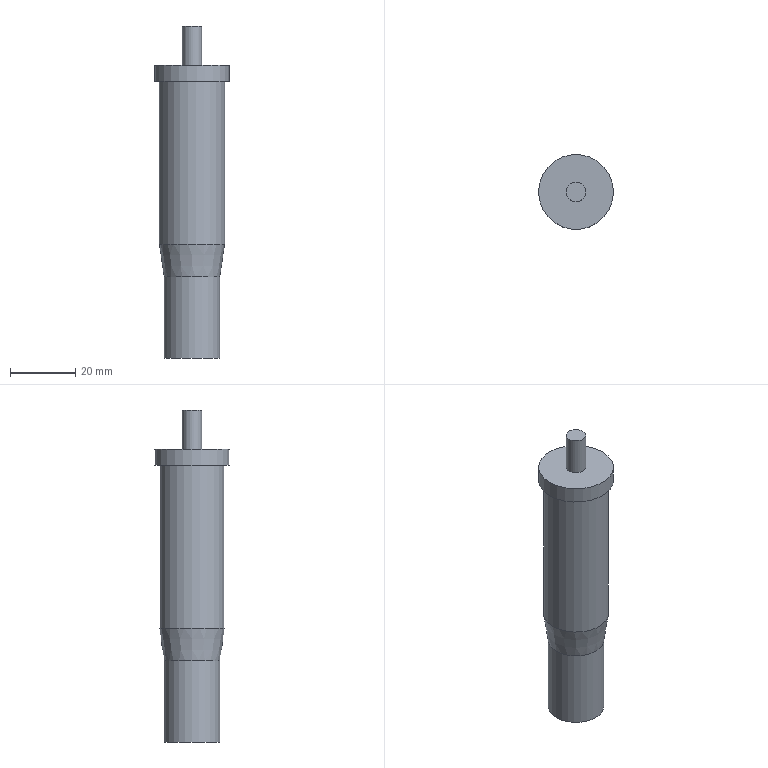Part | NX | features solid 2 | 1 solid | 9 faces | box 23 x 23 x 102 mm | volume 26574 mm3 | plane 4 | cylinder 4 | cone 1 | commonest cylinder face diameters 6 x1 17.1 x1 20 x1 23 x1
STEP:
#1=CARTESIAN_POINT('',(512.992,-137.822,-16.));
#2=VERTEX_POINT('',#1);
#3=CARTESIAN_POINT('',(521.542,-137.822,-16.));
#4=DIRECTION('',(0.,0.,-1.));
#5=DIRECTION('',(-1.,0.,0.));
#6=AXIS2_PLACEMENT_3D('',#3,#4,#5);
#7=CIRCLE('',#6,8.55);
#8=EDGE_CURVE('',#2,#2,#7,.T.);
#9=ORIENTED_EDGE('',*,*,#8,.T.);
#10=EDGE_LOOP('',(#9));
#11=FACE_BOUND('',#10,.T.);
#12=CARTESIAN_POINT('',(521.542,-137.822,-16.));
#13=DIRECTION('',(0.,0.,-1.));
#14=DIRECTION('',(1.,0.,0.));
#15=AXIS2_PLACEMENT_3D('',#12,#13,#14);
#16=PLANE('',#15);
#17=ADVANCED_FACE('',(#11),#16,.T.);
#18=CARTESIAN_POINT('',(512.992,-137.822,9.));
#19=VERTEX_POINT('',#18);
#20=CARTESIAN_POINT('',(521.542,-137.822,9.));
#21=DIRECTION('',(0.,0.,-1.));
#22=DIRECTION('',(-1.,0.,0.));
#23=AXIS2_PLACEMENT_3D('',#20,#21,#22);
#24=CIRCLE('',#23,8.55);
#25=EDGE_CURVE('',#19,#19,#24,.T.);
#26=ORIENTED_EDGE('',*,*,#25,.T.);
#27=EDGE_LOOP('',(#26));
#28=FACE_BOUND('',#27,.T.);
#29=ORIENTED_EDGE('',*,*,#8,.F.);
#30=EDGE_LOOP('',(#29));
#31=FACE_BOUND('',#30,.T.);
#32=CARTESIAN_POINT('',(521.542,-137.822,-16.));
#33=DIRECTION('',(0.,0.,1.));
#34=DIRECTION('',(-1.,0.,0.));
#35=AXIS2_PLACEMENT_3D('',#32,#33,#34);
#36=CYLINDRICAL_SURFACE('',#35,8.55);
#37=ADVANCED_FACE('',(#28,#31),#36,.T.);
#38=ORIENTED_EDGE('',*,*,#25,.F.);
#39=EDGE_LOOP('',(#38));
#40=FACE_BOUND('',#39,.T.);
#41=CARTESIAN_POINT('',(511.542,-137.822,19.));
#42=VERTEX_POINT('',#41);
#43=CARTESIAN_POINT('',(521.542,-137.822,19.));
#44=DIRECTION('',(0.,0.,-1.));
#45=DIRECTION('',(-1.,0.,0.));
#46=AXIS2_PLACEMENT_3D('',#43,#44,#45);
#47=CIRCLE('',#46,10.);
#48=EDGE_CURVE('',#42,#42,#47,.T.);
#49=ORIENTED_EDGE('',*,*,#48,.T.);
#50=EDGE_LOOP('',(#49));
#51=FACE_BOUND('',#50,.T.);
#52=CARTESIAN_POINT('',(521.542,-137.822,9.));
#53=DIRECTION('',(0.,0.,1.));
#54=DIRECTION('',(-1.,0.,0.));
#55=AXIS2_PLACEMENT_3D('',#52,#53,#54);
#56=CONICAL_SURFACE('',#55,8.55,0.144);
#57=ADVANCED_FACE('',(#40,#51),#56,.T.);
#58=CARTESIAN_POINT('',(531.542,-137.822,69.));
#59=VERTEX_POINT('',#58);
#60=CARTESIAN_POINT('',(521.542,-137.822,69.));
#61=DIRECTION('',(0.,0.,1.));
#62=DIRECTION('',(1.,0.,0.));
#63=AXIS2_PLACEMENT_3D('',#60,#61,#62);
#64=CIRCLE('',#63,10.);
#65=EDGE_CURVE('',#59,#59,#64,.F.);
#66=ORIENTED_EDGE('',*,*,#65,.T.);
#67=EDGE_LOOP('',(#66));
#68=FACE_BOUND('',#67,.T.);
#69=ORIENTED_EDGE('',*,*,#48,.F.);
#70=EDGE_LOOP('',(#69));
#71=FACE_BOUND('',#70,.T.);
#72=CARTESIAN_POINT('',(521.542,-137.822,19.));
#73=DIRECTION('',(0.,0.,1.));
#74=DIRECTION('',(-1.,0.,0.));
#75=AXIS2_PLACEMENT_3D('',#72,#73,#74);
#76=CYLINDRICAL_SURFACE('',#75,10.);
#77=ADVANCED_FACE('',(#68,#71),#76,.T.);
#78=CARTESIAN_POINT('',(518.542,-137.822,74.));
#79=VERTEX_POINT('',#78);
#80=CARTESIAN_POINT('',(521.542,-137.822,74.));
#81=DIRECTION('',(0.,0.,-1.));
#82=DIRECTION('',(-1.,0.,0.));
#83=AXIS2_PLACEMENT_3D('',#80,#81,#82);
#84=CIRCLE('',#83,3.);
#85=EDGE_CURVE('',#79,#79,#84,.T.);
#86=ORIENTED_EDGE('',*,*,#85,.T.);
#87=EDGE_LOOP('',(#86));
#88=FACE_BOUND('',#87,.T.);
#89=CARTESIAN_POINT('',(533.042,-137.822,74.));
#90=VERTEX_POINT('',#89);
#91=CARTESIAN_POINT('',(521.542,-137.822,74.));
#92=DIRECTION('',(0.,0.,1.));
#93=DIRECTION('',(1.,0.,0.));
#94=AXIS2_PLACEMENT_3D('',#91,#92,#93);
#95=CIRCLE('',#94,11.5);
#96=EDGE_CURVE('',#90,#90,#95,.T.);
#97=ORIENTED_EDGE('',*,*,#96,.T.);
#98=EDGE_LOOP('',(#97));
#99=FACE_BOUND('',#98,.T.);
#100=CARTESIAN_POINT('',(521.542,-137.822,74.));
#101=DIRECTION('',(0.,0.,1.));
#102=DIRECTION('',(-1.,0.,0.));
#103=AXIS2_PLACEMENT_3D('',#100,#101,#102);
#104=PLANE('',#103);
#105=ADVANCED_FACE('',(#88,#99),#104,.T.);
#106=ORIENTED_EDGE('',*,*,#65,.F.);
#107=EDGE_LOOP('',(#106));
#108=FACE_BOUND('',#107,.T.);
#109=CARTESIAN_POINT('',(510.042,-137.822,69.));
#110=VERTEX_POINT('',#109);
#111=CARTESIAN_POINT('',(521.542,-137.822,69.));
#112=DIRECTION('',(0.,0.,-1.));
#113=DIRECTION('',(-1.,0.,0.));
#114=AXIS2_PLACEMENT_3D('',#111,#112,#113);
#115=CIRCLE('',#114,11.5);
#116=EDGE_CURVE('',#110,#110,#115,.T.);
#117=ORIENTED_EDGE('',*,*,#116,.T.);
#118=EDGE_LOOP('',(#117));
#119=FACE_BOUND('',#118,.T.);
#120=CARTESIAN_POINT('',(521.542,-137.822,69.));
#121=DIRECTION('',(0.,0.,-1.));
#122=DIRECTION('',(1.,0.,0.));
#123=AXIS2_PLACEMENT_3D('',#120,#121,#122);
#124=PLANE('',#123);
#125=ADVANCED_FACE('',(#108,#119),#124,.T.);
#126=ORIENTED_EDGE('',*,*,#96,.F.);
#127=EDGE_LOOP('',(#126));
#128=FACE_BOUND('',#127,.T.);
#129=ORIENTED_EDGE('',*,*,#116,.F.);
#130=EDGE_LOOP('',(#129));
#131=FACE_BOUND('',#130,.T.);
#132=CARTESIAN_POINT('',(521.542,-137.822,69.));
#133=DIRECTION('',(0.,0.,1.));
#134=DIRECTION('',(-1.,0.,0.));
#135=AXIS2_PLACEMENT_3D('',#132,#133,#134);
#136=CYLINDRICAL_SURFACE('',#135,11.5);
#137=ADVANCED_FACE('',(#128,#131),#136,.T.);
#138=CARTESIAN_POINT('',(524.542,-137.822,86.));
#139=VERTEX_POINT('',#138);
#140=CARTESIAN_POINT('',(521.542,-137.822,86.));
#141=DIRECTION('',(0.,0.,1.));
#142=DIRECTION('',(1.,0.,0.));
#143=AXIS2_PLACEMENT_3D('',#140,#141,#142);
#144=CIRCLE('',#143,3.);
#145=EDGE_CURVE('',#139,#139,#144,.T.);
#146=ORIENTED_EDGE('',*,*,#145,.T.);
#147=EDGE_LOOP('',(#146));
#148=FACE_BOUND('',#147,.T.);
#149=CARTESIAN_POINT('',(521.542,-137.822,86.));
#150=DIRECTION('',(0.,0.,1.));
#151=DIRECTION('',(-1.,0.,0.));
#152=AXIS2_PLACEMENT_3D('',#149,#150,#151);
#153=PLANE('',#152);
#154=ADVANCED_FACE('',(#148),#153,.T.);
#155=ORIENTED_EDGE('',*,*,#145,.F.);
#156=EDGE_LOOP('',(#155));
#157=FACE_BOUND('',#156,.T.);
#158=ORIENTED_EDGE('',*,*,#85,.F.);
#159=EDGE_LOOP('',(#158));
#160=FACE_BOUND('',#159,.T.);
#161=CARTESIAN_POINT('',(521.542,-137.822,74.));
#162=DIRECTION('',(0.,0.,1.));
#163=DIRECTION('',(-1.,0.,0.));
#164=AXIS2_PLACEMENT_3D('',#161,#162,#163);
#165=CYLINDRICAL_SURFACE('',#164,3.);
#166=ADVANCED_FACE('',(#157,#160),#165,.T.);
#167=CLOSED_SHELL('',(#17,#37,#57,#77,#105,#125,#137,#154,#166));
#168=MANIFOLD_SOLID_BREP('',#167);
#169=(LENGTH_UNIT()NAMED_UNIT(*)SI_UNIT(.MILLI.,.METRE.));
#170=UNCERTAINTY_MEASURE_WITH_UNIT(LENGTH_MEASURE(0.00001),#169,'','');
#171=(NAMED_UNIT(*)PLANE_ANGLE_UNIT()SI_UNIT($,.RADIAN.));
#172=(NAMED_UNIT(*)SI_UNIT($,.STERADIAN.)SOLID_ANGLE_UNIT());
#173=(GEOMETRIC_REPRESENTATION_CONTEXT(3)GLOBAL_UNCERTAINTY_ASSIGNED_CONTEXT((#170))GLOBAL_UNIT_ASSIGNED_CONTEXT((#169,#171,#172))REPRESENTATION_CONTEXT('',''));
#174=ADVANCED_BREP_SHAPE_REPRESENTATION('',(#168),#173);